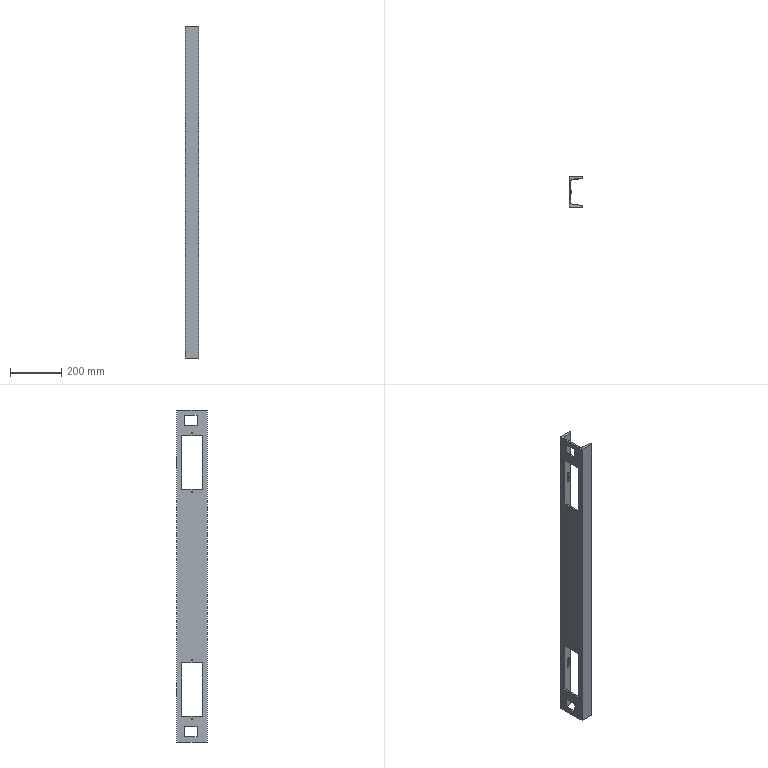Part | SolidWorks | features BaseBody 1 | 1 solid | 88 faces | box 53 x 120 x 1300 mm | volume 1778811 mm3 | plane 62 | cylinder 26 | commonest cylinder face diameters 5 x8 5.5 x8 15 x6 9 x2 18 x2